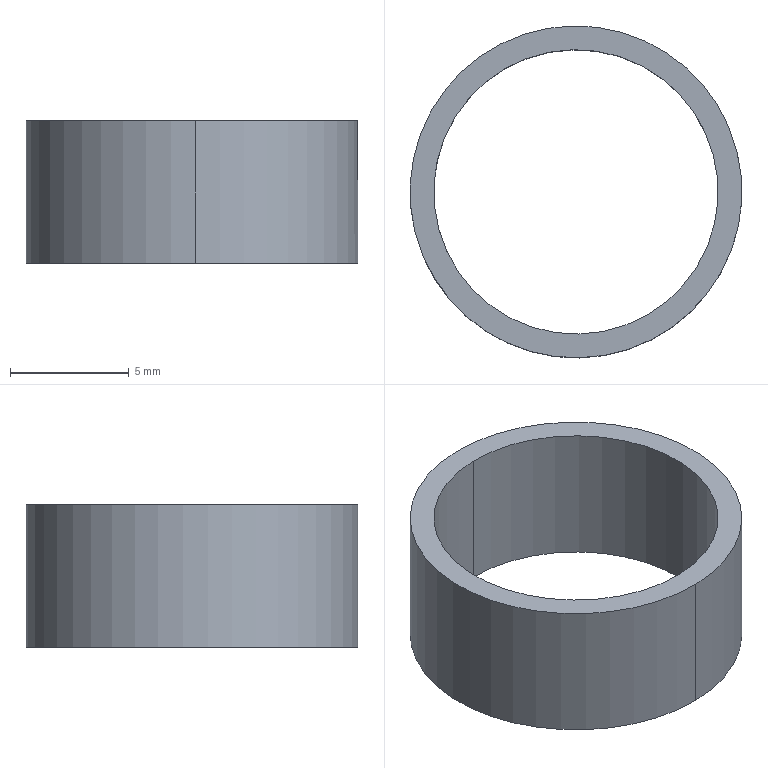Part | SolidWorks | features BaseBody 1 | 1 solid | 6 faces | box 14.001 x 14 x 6.002 mm | volume 245.044 mm3 | cylinder 4 | plane 2 | commonest cylinder face diameters 12 x2 14 x2
STEP:
#1=CARTESIAN_POINT('',(418.143,218.515,13.486));
#2=VERTEX_POINT('',#1);
#3=CARTESIAN_POINT('',(418.395,206.518,13.486));
#4=VERTEX_POINT('',#3);
#5=CARTESIAN_POINT('',(418.269,212.516,13.486));
#6=DIRECTION('',(0.0001435,0.000000521,-1.));
#7=DIRECTION('',(-0.02104,0.9998,-0.000002497));
#8=AXIS2_PLACEMENT_3D('',#5,#6,#7);
#9=CIRCLE('',#8,6.);
#10=EDGE_CURVE('',#2,#4,#9,.T.);
#11=ORIENTED_EDGE('',*,*,#10,.F.);
#12=CARTESIAN_POINT('',(418.143,218.515,7.486));
#13=VERTEX_POINT('',#12);
#14=CARTESIAN_POINT('',(418.142,218.515,15.486));
#15=DIRECTION('',(0.0001435,0.000000521,-1.));
#16=VECTOR('',#15,1000.);
#17=LINE('',#14,#16);
#18=EDGE_CURVE('',#2,#13,#17,.T.);
#19=ORIENTED_EDGE('',*,*,#18,.T.);
#20=CARTESIAN_POINT('',(418.396,206.518,7.486));
#21=VERTEX_POINT('',#20);
#22=CARTESIAN_POINT('',(418.27,212.516,7.486));
#23=DIRECTION('',(-0.0001435,-0.000000521,1.));
#24=DIRECTION('',(-1.,0.,-0.0001435));
#25=AXIS2_PLACEMENT_3D('',#22,#23,#24);
#26=CIRCLE('',#25,6.);
#27=EDGE_CURVE('',#21,#13,#26,.T.);
#28=ORIENTED_EDGE('',*,*,#27,.F.);
#29=CARTESIAN_POINT('',(418.395,206.518,15.486));
#30=DIRECTION('',(0.0001435,0.000000521,-1.));
#31=VECTOR('',#30,1000.);
#32=LINE('',#29,#31);
#33=EDGE_CURVE('',#4,#21,#32,.T.);
#34=ORIENTED_EDGE('',*,*,#33,.F.);
#35=EDGE_LOOP('',(#11,#19,#28,#34));
#36=FACE_OUTER_BOUND('',#35,.T.);
#37=CARTESIAN_POINT('',(418.269,212.516,15.486));
#38=DIRECTION('',(0.0001435,0.000000521,-1.));
#39=DIRECTION('',(0.02104,-0.9998,0.000002497));
#40=AXIS2_PLACEMENT_3D('',#37,#38,#39);
#41=CYLINDRICAL_SURFACE('',#40,6.);
#42=ADVANCED_FACE('',(#36),#41,.F.);
#43=CARTESIAN_POINT('',(418.122,219.515,13.486));
#44=VERTEX_POINT('',#43);
#45=CARTESIAN_POINT('',(418.416,205.518,13.486));
#46=VERTEX_POINT('',#45);
#47=CARTESIAN_POINT('',(418.269,212.516,13.486));
#48=DIRECTION('',(-0.0001435,-0.000000521,1.));
#49=DIRECTION('',(-0.02104,0.9998,-0.000002497));
#50=AXIS2_PLACEMENT_3D('',#47,#48,#49);
#51=CIRCLE('',#50,7.);
#52=EDGE_CURVE('',#44,#46,#51,.T.);
#53=ORIENTED_EDGE('',*,*,#52,.F.);
#54=CARTESIAN_POINT('',(418.122,219.515,7.486));
#55=VERTEX_POINT('',#54);
#56=CARTESIAN_POINT('',(418.121,219.515,15.486));
#57=DIRECTION('',(0.0001435,0.000000521,-1.));
#58=VECTOR('',#57,1000.);
#59=LINE('',#56,#58);
#60=EDGE_CURVE('',#44,#55,#59,.T.);
#61=ORIENTED_EDGE('',*,*,#60,.T.);
#62=CARTESIAN_POINT('',(418.417,205.518,7.486));
#63=VERTEX_POINT('',#62);
#64=CARTESIAN_POINT('',(418.27,212.516,7.486));
#65=DIRECTION('',(0.0001435,0.000000521,-1.));
#66=DIRECTION('',(0.02104,-0.9998,0.000002497));
#67=AXIS2_PLACEMENT_3D('',#64,#65,#66);
#68=CIRCLE('',#67,7.);
#69=EDGE_CURVE('',#63,#55,#68,.T.);
#70=ORIENTED_EDGE('',*,*,#69,.F.);
#71=CARTESIAN_POINT('',(418.416,205.518,15.486));
#72=DIRECTION('',(0.0001435,0.000000521,-1.));
#73=VECTOR('',#72,1000.);
#74=LINE('',#71,#73);
#75=EDGE_CURVE('',#46,#63,#74,.T.);
#76=ORIENTED_EDGE('',*,*,#75,.F.);
#77=EDGE_LOOP('',(#53,#61,#70,#76));
#78=FACE_OUTER_BOUND('',#77,.T.);
#79=CARTESIAN_POINT('',(418.269,212.516,15.486));
#80=DIRECTION('',(0.0001435,0.000000521,-1.));
#81=DIRECTION('',(0.02104,-0.9998,0.000002497));
#82=AXIS2_PLACEMENT_3D('',#79,#80,#81);
#83=CYLINDRICAL_SURFACE('',#82,7.);
#84=ADVANCED_FACE('',(#78),#83,.T.);
#85=ORIENTED_EDGE('',*,*,#60,.F.);
#86=CARTESIAN_POINT('',(418.269,212.516,13.486));
#87=DIRECTION('',(-0.0001435,-0.000000521,1.));
#88=DIRECTION('',(-0.02104,0.9998,-0.000002497));
#89=AXIS2_PLACEMENT_3D('',#86,#87,#88);
#90=CIRCLE('',#89,7.);
#91=EDGE_CURVE('',#46,#44,#90,.T.);
#92=ORIENTED_EDGE('',*,*,#91,.F.);
#93=ORIENTED_EDGE('',*,*,#75,.T.);
#94=CARTESIAN_POINT('',(418.27,212.516,7.486));
#95=DIRECTION('',(0.0001435,0.000000521,-1.));
#96=DIRECTION('',(0.02104,-0.9998,0.000002497));
#97=AXIS2_PLACEMENT_3D('',#94,#95,#96);
#98=CIRCLE('',#97,7.);
#99=EDGE_CURVE('',#55,#63,#98,.T.);
#100=ORIENTED_EDGE('',*,*,#99,.F.);
#101=EDGE_LOOP('',(#85,#92,#93,#100));
#102=FACE_OUTER_BOUND('',#101,.T.);
#103=CARTESIAN_POINT('',(418.269,212.516,15.486));
#104=DIRECTION('',(0.0001435,0.000000521,-1.));
#105=DIRECTION('',(0.02104,-0.9998,0.000002497));
#106=AXIS2_PLACEMENT_3D('',#103,#104,#105);
#107=CYLINDRICAL_SURFACE('',#106,7.);
#108=ADVANCED_FACE('',(#102),#107,.T.);
#109=ORIENTED_EDGE('',*,*,#27,.T.);
#110=CARTESIAN_POINT('',(418.27,212.516,7.486));
#111=DIRECTION('',(-0.0001435,-0.000000521,1.));
#112=DIRECTION('',(-1.,0.,-0.0001435));
#113=AXIS2_PLACEMENT_3D('',#110,#111,#112);
#114=CIRCLE('',#113,6.);
#115=EDGE_CURVE('',#13,#21,#114,.T.);
#116=ORIENTED_EDGE('',*,*,#115,.T.);
#117=EDGE_LOOP('',(#109,#116));
#118=FACE_BOUND('',#117,.T.);
#119=ORIENTED_EDGE('',*,*,#69,.T.);
#120=ORIENTED_EDGE('',*,*,#99,.T.);
#121=EDGE_LOOP('',(#119,#120));
#122=FACE_OUTER_BOUND('',#121,.T.);
#123=CARTESIAN_POINT('',(418.27,212.516,7.486));
#124=DIRECTION('',(0.0001435,0.000000521,-1.));
#125=DIRECTION('',(0.,-1.,-0.000000521));
#126=AXIS2_PLACEMENT_3D('',#123,#124,#125);
#127=PLANE('',#126);
#128=ADVANCED_FACE('',(#118,#122),#127,.T.);
#129=ORIENTED_EDGE('',*,*,#18,.F.);
#130=CARTESIAN_POINT('',(418.269,212.516,13.486));
#131=DIRECTION('',(0.0001435,0.000000521,-1.));
#132=DIRECTION('',(-0.02104,0.9998,-0.000002497));
#133=AXIS2_PLACEMENT_3D('',#130,#131,#132);
#134=CIRCLE('',#133,6.);
#135=EDGE_CURVE('',#4,#2,#134,.T.);
#136=ORIENTED_EDGE('',*,*,#135,.F.);
#137=ORIENTED_EDGE('',*,*,#33,.T.);
#138=ORIENTED_EDGE('',*,*,#115,.F.);
#139=EDGE_LOOP('',(#129,#136,#137,#138));
#140=FACE_OUTER_BOUND('',#139,.T.);
#141=CARTESIAN_POINT('',(418.269,212.516,15.486));
#142=DIRECTION('',(0.0001435,0.000000521,-1.));
#143=DIRECTION('',(0.02104,-0.9998,0.000002497));
#144=AXIS2_PLACEMENT_3D('',#141,#142,#143);
#145=CYLINDRICAL_SURFACE('',#144,6.);
#146=ADVANCED_FACE('',(#140),#145,.F.);
#147=ORIENTED_EDGE('',*,*,#135,.T.);
#148=ORIENTED_EDGE('',*,*,#10,.T.);
#149=EDGE_LOOP('',(#147,#148));
#150=FACE_BOUND('',#149,.T.);
#151=ORIENTED_EDGE('',*,*,#91,.T.);
#152=ORIENTED_EDGE('',*,*,#52,.T.);
#153=EDGE_LOOP('',(#151,#152));
#154=FACE_OUTER_BOUND('',#153,.T.);
#155=CARTESIAN_POINT('',(418.269,212.516,13.486));
#156=DIRECTION('',(0.0001435,0.000000521,-1.));
#157=DIRECTION('',(0.,-1.,-0.000000521));
#158=AXIS2_PLACEMENT_3D('',#155,#156,#157);
#159=PLANE('',#158);
#160=ADVANCED_FACE('',(#150,#154),#159,.F.);
#161=CLOSED_SHELL('',(#42,#84,#108,#128,#146,#160));
#162=MANIFOLD_SOLID_BREP('',#161);
#163=CARTESIAN_POINT('',(0.,0.,0.));
#164=DIRECTION('',(0.,0.,1.));
#165=DIRECTION('',(1.,0.,0.));
#166=AXIS2_PLACEMENT_3D('',#163,#164,#165);
#167=(LENGTH_UNIT()NAMED_UNIT(*)SI_UNIT(.MILLI.,.METRE.));
#168=UNCERTAINTY_MEASURE_WITH_UNIT(LENGTH_MEASURE(0.00001),#167,'','');
#169=(NAMED_UNIT(*)PLANE_ANGLE_UNIT()SI_UNIT($,.RADIAN.));
#170=(NAMED_UNIT(*)SI_UNIT($,.STERADIAN.)SOLID_ANGLE_UNIT());
#171=(GEOMETRIC_REPRESENTATION_CONTEXT(3)GLOBAL_UNCERTAINTY_ASSIGNED_CONTEXT((#168))GLOBAL_UNIT_ASSIGNED_CONTEXT((#167,#169,#170))REPRESENTATION_CONTEXT('',''));
#172=ADVANCED_BREP_SHAPE_REPRESENTATION('',(#162,#166),#171);